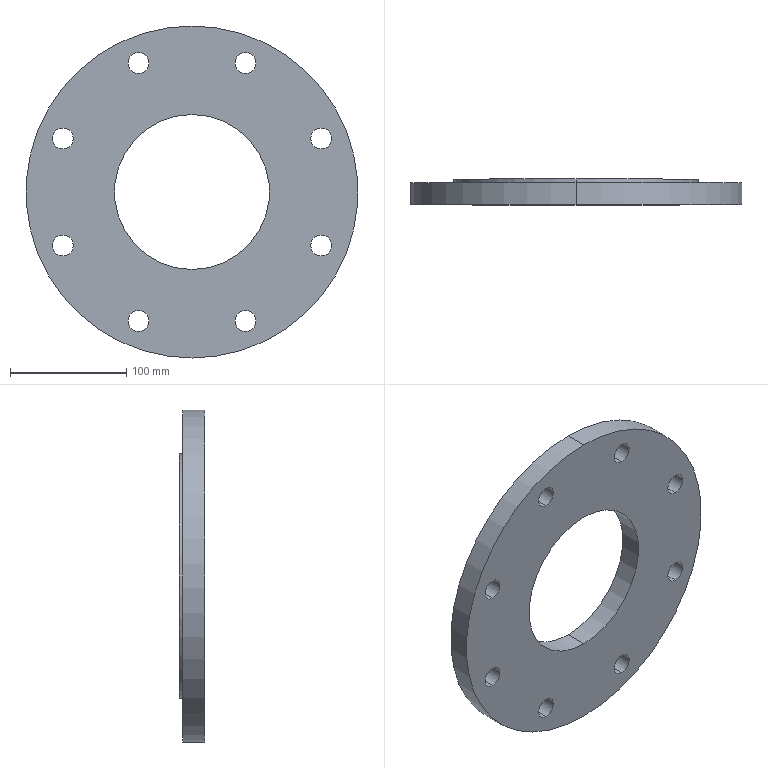Part | SolidWorks | features ICE 2, CirPattern 1, Extrusion 1 | 1 solid | 28 faces | box 285 x 22 x 285 mm | volume 945255 mm3 | cylinder 24 | plane 4 | commonest cylinder face diameters 18 x16 133 x2 170 x2 210 x2 285 x2
STEP:
#1=CARTESIAN_POINT('',(45.922,-9.5,-119.866));
#2=VERTEX_POINT('',#1);
#3=CARTESIAN_POINT('',(45.922,-9.5,-101.866));
#4=VERTEX_POINT('',#3);
#5=CARTESIAN_POINT('',(45.922,-9.5,-110.866));
#6=DIRECTION('',(0.,1.,0.));
#7=DIRECTION('',(-0.7071,0.,0.7071));
#8=AXIS2_PLACEMENT_3D('',#5,#6,#7);
#9=CIRCLE('',#8,9.);
#10=EDGE_CURVE('',#2,#4,#9,.T.);
#11=ORIENTED_EDGE('',*,*,#10,.F.);
#12=CARTESIAN_POINT('',(45.922,9.5,-119.866));
#13=VERTEX_POINT('',#12);
#14=CARTESIAN_POINT('',(45.922,-9.5,-119.866));
#15=DIRECTION('',(0.,1.,0.));
#16=VECTOR('',#15,1000.);
#17=LINE('',#14,#16);
#18=EDGE_CURVE('',#2,#13,#17,.T.);
#19=ORIENTED_EDGE('',*,*,#18,.T.);
#20=CARTESIAN_POINT('',(45.922,9.5,-101.866));
#21=VERTEX_POINT('',#20);
#22=CARTESIAN_POINT('',(45.922,9.5,-110.866));
#23=DIRECTION('',(0.,1.,0.));
#24=DIRECTION('',(-0.7071,0.,0.7071));
#25=AXIS2_PLACEMENT_3D('',#22,#23,#24);
#26=CIRCLE('',#25,9.);
#27=EDGE_CURVE('',#13,#21,#26,.T.);
#28=ORIENTED_EDGE('',*,*,#27,.T.);
#29=CARTESIAN_POINT('',(45.922,-9.5,-101.866));
#30=DIRECTION('',(0.,1.,0.));
#31=VECTOR('',#30,1000.);
#32=LINE('',#29,#31);
#33=EDGE_CURVE('',#4,#21,#32,.T.);
#34=ORIENTED_EDGE('',*,*,#33,.F.);
#35=EDGE_LOOP('',(#11,#19,#28,#34));
#36=FACE_OUTER_BOUND('',#35,.T.);
#37=CARTESIAN_POINT('',(45.922,-9.5,-110.866));
#38=DIRECTION('',(0.,1.,0.));
#39=DIRECTION('',(0.,0.,1.));
#40=AXIS2_PLACEMENT_3D('',#37,#38,#39);
#41=CYLINDRICAL_SURFACE('',#40,9.);
#42=ADVANCED_FACE('',(#36),#41,.F.);
#43=CARTESIAN_POINT('',(110.866,-9.5,-54.922));
#44=VERTEX_POINT('',#43);
#45=CARTESIAN_POINT('',(110.866,-9.5,-36.922));
#46=VERTEX_POINT('',#45);
#47=CARTESIAN_POINT('',(110.866,-9.5,-45.922));
#48=DIRECTION('',(0.,1.,0.));
#49=DIRECTION('',(-1.,0.,0.));
#50=AXIS2_PLACEMENT_3D('',#47,#48,#49);
#51=CIRCLE('',#50,9.);
#52=EDGE_CURVE('',#44,#46,#51,.T.);
#53=ORIENTED_EDGE('',*,*,#52,.F.);
#54=CARTESIAN_POINT('',(110.866,9.5,-54.922));
#55=VERTEX_POINT('',#54);
#56=CARTESIAN_POINT('',(110.866,-9.5,-54.922));
#57=DIRECTION('',(0.,1.,0.));
#58=VECTOR('',#57,1000.);
#59=LINE('',#56,#58);
#60=EDGE_CURVE('',#44,#55,#59,.T.);
#61=ORIENTED_EDGE('',*,*,#60,.T.);
#62=CARTESIAN_POINT('',(110.866,9.5,-36.922));
#63=VERTEX_POINT('',#62);
#64=CARTESIAN_POINT('',(110.866,9.5,-45.922));
#65=DIRECTION('',(0.,1.,0.));
#66=DIRECTION('',(-1.,0.,0.));
#67=AXIS2_PLACEMENT_3D('',#64,#65,#66);
#68=CIRCLE('',#67,9.);
#69=EDGE_CURVE('',#55,#63,#68,.T.);
#70=ORIENTED_EDGE('',*,*,#69,.T.);
#71=CARTESIAN_POINT('',(110.866,-9.5,-36.922));
#72=DIRECTION('',(0.,1.,0.));
#73=VECTOR('',#72,1000.);
#74=LINE('',#71,#73);
#75=EDGE_CURVE('',#46,#63,#74,.T.);
#76=ORIENTED_EDGE('',*,*,#75,.F.);
#77=EDGE_LOOP('',(#53,#61,#70,#76));
#78=FACE_OUTER_BOUND('',#77,.T.);
#79=CARTESIAN_POINT('',(110.866,-9.5,-45.922));
#80=DIRECTION('',(0.,1.,0.));
#81=DIRECTION('',(0.,0.,1.));
#82=AXIS2_PLACEMENT_3D('',#79,#80,#81);
#83=CYLINDRICAL_SURFACE('',#82,9.);
#84=ADVANCED_FACE('',(#78),#83,.F.);
#85=CARTESIAN_POINT('',(110.866,-9.5,36.922));
#86=VERTEX_POINT('',#85);
#87=CARTESIAN_POINT('',(110.866,-9.5,54.922));
#88=VERTEX_POINT('',#87);
#89=CARTESIAN_POINT('',(110.866,-9.5,45.922));
#90=DIRECTION('',(0.,1.,0.));
#91=DIRECTION('',(-0.7071,0.,-0.7071));
#92=AXIS2_PLACEMENT_3D('',#89,#90,#91);
#93=CIRCLE('',#92,9.);
#94=EDGE_CURVE('',#86,#88,#93,.T.);
#95=ORIENTED_EDGE('',*,*,#94,.F.);
#96=CARTESIAN_POINT('',(110.866,9.5,36.922));
#97=VERTEX_POINT('',#96);
#98=CARTESIAN_POINT('',(110.866,-9.5,36.922));
#99=DIRECTION('',(0.,1.,0.));
#100=VECTOR('',#99,1000.);
#101=LINE('',#98,#100);
#102=EDGE_CURVE('',#86,#97,#101,.T.);
#103=ORIENTED_EDGE('',*,*,#102,.T.);
#104=CARTESIAN_POINT('',(110.866,9.5,54.922));
#105=VERTEX_POINT('',#104);
#106=CARTESIAN_POINT('',(110.866,9.5,45.922));
#107=DIRECTION('',(0.,1.,0.));
#108=DIRECTION('',(-0.7071,0.,-0.7071));
#109=AXIS2_PLACEMENT_3D('',#106,#107,#108);
#110=CIRCLE('',#109,9.);
#111=EDGE_CURVE('',#97,#105,#110,.T.);
#112=ORIENTED_EDGE('',*,*,#111,.T.);
#113=CARTESIAN_POINT('',(110.866,-9.5,54.922));
#114=DIRECTION('',(0.,1.,0.));
#115=VECTOR('',#114,1000.);
#116=LINE('',#113,#115);
#117=EDGE_CURVE('',#88,#105,#116,.T.);
#118=ORIENTED_EDGE('',*,*,#117,.F.);
#119=EDGE_LOOP('',(#95,#103,#112,#118));
#120=FACE_OUTER_BOUND('',#119,.T.);
#121=CARTESIAN_POINT('',(110.866,-9.5,45.922));
#122=DIRECTION('',(0.,1.,0.));
#123=DIRECTION('',(0.,0.,1.));
#124=AXIS2_PLACEMENT_3D('',#121,#122,#123);
#125=CYLINDRICAL_SURFACE('',#124,9.);
#126=ADVANCED_FACE('',(#120),#125,.F.);
#127=CARTESIAN_POINT('',(45.922,-9.5,101.866));
#128=VERTEX_POINT('',#127);
#129=CARTESIAN_POINT('',(45.922,-9.5,119.866));
#130=VERTEX_POINT('',#129);
#131=CARTESIAN_POINT('',(45.922,-9.5,110.866));
#132=DIRECTION('',(0.,1.,0.));
#133=DIRECTION('',(0.,0.,-1.));
#134=AXIS2_PLACEMENT_3D('',#131,#132,#133);
#135=CIRCLE('',#134,9.);
#136=EDGE_CURVE('',#128,#130,#135,.T.);
#137=ORIENTED_EDGE('',*,*,#136,.F.);
#138=CARTESIAN_POINT('',(45.922,9.5,101.866));
#139=VERTEX_POINT('',#138);
#140=CARTESIAN_POINT('',(45.922,-9.5,101.866));
#141=DIRECTION('',(0.,1.,0.));
#142=VECTOR('',#141,1000.);
#143=LINE('',#140,#142);
#144=EDGE_CURVE('',#128,#139,#143,.T.);
#145=ORIENTED_EDGE('',*,*,#144,.T.);
#146=CARTESIAN_POINT('',(45.922,9.5,119.866));
#147=VERTEX_POINT('',#146);
#148=CARTESIAN_POINT('',(45.922,9.5,110.866));
#149=DIRECTION('',(0.,1.,0.));
#150=DIRECTION('',(0.,0.,-1.));
#151=AXIS2_PLACEMENT_3D('',#148,#149,#150);
#152=CIRCLE('',#151,9.);
#153=EDGE_CURVE('',#139,#147,#152,.T.);
#154=ORIENTED_EDGE('',*,*,#153,.T.);
#155=CARTESIAN_POINT('',(45.922,-9.5,119.866));
#156=DIRECTION('',(0.,1.,0.));
#157=VECTOR('',#156,1000.);
#158=LINE('',#155,#157);
#159=EDGE_CURVE('',#130,#147,#158,.T.);
#160=ORIENTED_EDGE('',*,*,#159,.F.);
#161=EDGE_LOOP('',(#137,#145,#154,#160));
#162=FACE_OUTER_BOUND('',#161,.T.);
#163=CARTESIAN_POINT('',(45.922,-9.5,110.866));
#164=DIRECTION('',(0.,1.,0.));
#165=DIRECTION('',(0.,0.,1.));
#166=AXIS2_PLACEMENT_3D('',#163,#164,#165);
#167=CYLINDRICAL_SURFACE('',#166,9.);
#168=ADVANCED_FACE('',(#162),#167,.F.);
#169=CARTESIAN_POINT('',(-45.922,-9.5,101.866));
#170=VERTEX_POINT('',#169);
#171=CARTESIAN_POINT('',(-45.922,-9.5,119.866));
#172=VERTEX_POINT('',#171);
#173=CARTESIAN_POINT('',(-45.922,-9.5,110.866));
#174=DIRECTION('',(0.,1.,0.));
#175=DIRECTION('',(0.7071,0.,-0.7071));
#176=AXIS2_PLACEMENT_3D('',#173,#174,#175);
#177=CIRCLE('',#176,9.);
#178=EDGE_CURVE('',#170,#172,#177,.T.);
#179=ORIENTED_EDGE('',*,*,#178,.F.);
#180=CARTESIAN_POINT('',(-45.922,9.5,101.866));
#181=VERTEX_POINT('',#180);
#182=CARTESIAN_POINT('',(-45.922,-9.5,101.866));
#183=DIRECTION('',(0.,1.,0.));
#184=VECTOR('',#183,1000.);
#185=LINE('',#182,#184);
#186=EDGE_CURVE('',#170,#181,#185,.T.);
#187=ORIENTED_EDGE('',*,*,#186,.T.);
#188=CARTESIAN_POINT('',(-45.922,9.5,119.866));
#189=VERTEX_POINT('',#188);
#190=CARTESIAN_POINT('',(-45.922,9.5,110.866));
#191=DIRECTION('',(0.,1.,0.));
#192=DIRECTION('',(0.7071,0.,-0.7071));
#193=AXIS2_PLACEMENT_3D('',#190,#191,#192);
#194=CIRCLE('',#193,9.);
#195=EDGE_CURVE('',#181,#189,#194,.T.);
#196=ORIENTED_EDGE('',*,*,#195,.T.);
#197=CARTESIAN_POINT('',(-45.922,-9.5,119.866));
#198=DIRECTION('',(0.,1.,0.));
#199=VECTOR('',#198,1000.);
#200=LINE('',#197,#199);
#201=EDGE_CURVE('',#172,#189,#200,.T.);
#202=ORIENTED_EDGE('',*,*,#201,.F.);
#203=EDGE_LOOP('',(#179,#187,#196,#202));
#204=FACE_OUTER_BOUND('',#203,.T.);
#205=CARTESIAN_POINT('',(-45.922,-9.5,110.866));
#206=DIRECTION('',(0.,1.,0.));
#207=DIRECTION('',(0.,0.,1.));
#208=AXIS2_PLACEMENT_3D('',#205,#206,#207);
#209=CYLINDRICAL_SURFACE('',#208,9.);
#210=ADVANCED_FACE('',(#204),#209,.F.);
#211=CARTESIAN_POINT('',(-110.866,-9.5,36.922));
#212=VERTEX_POINT('',#211);
#213=CARTESIAN_POINT('',(-110.866,-9.5,54.922));
#214=VERTEX_POINT('',#213);
#215=CARTESIAN_POINT('',(-110.866,-9.5,45.922));
#216=DIRECTION('',(0.,1.,0.));
#217=DIRECTION('',(1.,0.,0.));
#218=AXIS2_PLACEMENT_3D('',#215,#216,#217);
#219=CIRCLE('',#218,9.);
#220=EDGE_CURVE('',#212,#214,#219,.T.);
#221=ORIENTED_EDGE('',*,*,#220,.F.);
#222=CARTESIAN_POINT('',(-110.866,9.5,36.922));
#223=VERTEX_POINT('',#222);
#224=CARTESIAN_POINT('',(-110.866,-9.5,36.922));
#225=DIRECTION('',(0.,1.,0.));
#226=VECTOR('',#225,1000.);
#227=LINE('',#224,#226);
#228=EDGE_CURVE('',#212,#223,#227,.T.);
#229=ORIENTED_EDGE('',*,*,#228,.T.);
#230=CARTESIAN_POINT('',(-110.866,9.5,54.922));
#231=VERTEX_POINT('',#230);
#232=CARTESIAN_POINT('',(-110.866,9.5,45.922));
#233=DIRECTION('',(0.,1.,0.));
#234=DIRECTION('',(1.,0.,0.));
#235=AXIS2_PLACEMENT_3D('',#232,#233,#234);
#236=CIRCLE('',#235,9.);
#237=EDGE_CURVE('',#223,#231,#236,.T.);
#238=ORIENTED_EDGE('',*,*,#237,.T.);
#239=CARTESIAN_POINT('',(-110.866,-9.5,54.922));
#240=DIRECTION('',(0.,1.,0.));
#241=VECTOR('',#240,1000.);
#242=LINE('',#239,#241);
#243=EDGE_CURVE('',#214,#231,#242,.T.);
#244=ORIENTED_EDGE('',*,*,#243,.F.);
#245=EDGE_LOOP('',(#221,#229,#238,#244));
#246=FACE_OUTER_BOUND('',#245,.T.);
#247=CARTESIAN_POINT('',(-110.866,-9.5,45.922));
#248=DIRECTION('',(0.,1.,0.));
#249=DIRECTION('',(0.,0.,1.));
#250=AXIS2_PLACEMENT_3D('',#247,#248,#249);
#251=CYLINDRICAL_SURFACE('',#250,9.);
#252=ADVANCED_FACE('',(#246),#251,.F.);
#253=CARTESIAN_POINT('',(-110.866,-9.5,-54.922));
#254=VERTEX_POINT('',#253);
#255=CARTESIAN_POINT('',(-110.866,-9.5,-36.922));
#256=VERTEX_POINT('',#255);
#257=CARTESIAN_POINT('',(-110.866,-9.5,-45.922));
#258=DIRECTION('',(0.,1.,0.));
#259=DIRECTION('',(0.7071,0.,0.7071));
#260=AXIS2_PLACEMENT_3D('',#257,#258,#259);
#261=CIRCLE('',#260,9.);
#262=EDGE_CURVE('',#254,#256,#261,.T.);
#263=ORIENTED_EDGE('',*,*,#262,.F.);
#264=CARTESIAN_POINT('',(-110.866,9.5,-54.922));
#265=VERTEX_POINT('',#264);
#266=CARTESIAN_POINT('',(-110.866,-9.5,-54.922));
#267=DIRECTION('',(0.,1.,0.));
#268=VECTOR('',#267,1000.);
#269=LINE('',#266,#268);
#270=EDGE_CURVE('',#254,#265,#269,.T.);
#271=ORIENTED_EDGE('',*,*,#270,.T.);
#272=CARTESIAN_POINT('',(-110.866,9.5,-36.922));
#273=VERTEX_POINT('',#272);
#274=CARTESIAN_POINT('',(-110.866,9.5,-45.922));
#275=DIRECTION('',(0.,1.,0.));
#276=DIRECTION('',(0.7071,0.,0.7071));
#277=AXIS2_PLACEMENT_3D('',#274,#275,#276);
#278=CIRCLE('',#277,9.);
#279=EDGE_CURVE('',#265,#273,#278,.T.);
#280=ORIENTED_EDGE('',*,*,#279,.T.);
#281=CARTESIAN_POINT('',(-110.866,-9.5,-36.922));
#282=DIRECTION('',(0.,1.,0.));
#283=VECTOR('',#282,1000.);
#284=LINE('',#281,#283);
#285=EDGE_CURVE('',#256,#273,#284,.T.);
#286=ORIENTED_EDGE('',*,*,#285,.F.);
#287=EDGE_LOOP('',(#263,#271,#280,#286));
#288=FACE_OUTER_BOUND('',#287,.T.);
#289=CARTESIAN_POINT('',(-110.866,-9.5,-45.922));
#290=DIRECTION('',(0.,1.,0.));
#291=DIRECTION('',(0.,0.,1.));
#292=AXIS2_PLACEMENT_3D('',#289,#290,#291);
#293=CYLINDRICAL_SURFACE('',#292,9.);
#294=ADVANCED_FACE('',(#288),#293,.F.);
#295=CARTESIAN_POINT('',(-45.922,-9.5,-119.866));
#296=VERTEX_POINT('',#295);
#297=CARTESIAN_POINT('',(-45.922,-9.5,-101.866));
#298=VERTEX_POINT('',#297);
#299=CARTESIAN_POINT('',(-45.922,-9.5,-110.866));
#300=DIRECTION('',(0.,1.,0.));
#301=DIRECTION('',(0.,0.,1.));
#302=AXIS2_PLACEMENT_3D('',#299,#300,#301);
#303=CIRCLE('',#302,9.);
#304=EDGE_CURVE('',#296,#298,#303,.T.);
#305=ORIENTED_EDGE('',*,*,#304,.F.);
#306=CARTESIAN_POINT('',(-45.922,9.5,-119.866));
#307=VERTEX_POINT('',#306);
#308=CARTESIAN_POINT('',(-45.922,-9.5,-119.866));
#309=DIRECTION('',(0.,1.,0.));
#310=VECTOR('',#309,1000.);
#311=LINE('',#308,#310);
#312=EDGE_CURVE('',#296,#307,#311,.T.);
#313=ORIENTED_EDGE('',*,*,#312,.T.);
#314=CARTESIAN_POINT('',(-45.922,9.5,-101.866));
#315=VERTEX_POINT('',#314);
#316=CARTESIAN_POINT('',(-45.922,9.5,-110.866));
#317=DIRECTION('',(0.,1.,0.));
#318=DIRECTION('',(0.,0.,1.));
#319=AXIS2_PLACEMENT_3D('',#316,#317,#318);
#320=CIRCLE('',#319,9.);
#321=EDGE_CURVE('',#307,#315,#320,.T.);
#322=ORIENTED_EDGE('',*,*,#321,.T.);
#323=CARTESIAN_POINT('',(-45.922,-9.5,-101.866));
#324=DIRECTION('',(0.,1.,0.));
#325=VECTOR('',#324,1000.);
#326=LINE('',#323,#325);
#327=EDGE_CURVE('',#298,#315,#326,.T.);
#328=ORIENTED_EDGE('',*,*,#327,.F.);
#329=EDGE_LOOP('',(#305,#313,#322,#328));
#330=FACE_OUTER_BOUND('',#329,.T.);
#331=CARTESIAN_POINT('',(-45.922,-9.5,-110.866));
#332=DIRECTION('',(0.,1.,0.));
#333=DIRECTION('',(0.,0.,1.));
#334=AXIS2_PLACEMENT_3D('',#331,#332,#333);
#335=CYLINDRICAL_SURFACE('',#334,9.);
#336=ADVANCED_FACE('',(#330),#335,.F.);
#337=CARTESIAN_POINT('',(0.,12.5,-85.));
#338=VERTEX_POINT('',#337);
#339=CARTESIAN_POINT('',(0.,12.5,85.));
#340=VERTEX_POINT('',#339);
#341=CARTESIAN_POINT('',(0.,12.5,0.));
#342=DIRECTION('',(0.,1.,0.));
#343=DIRECTION('',(0.,0.,1.));
#344=AXIS2_PLACEMENT_3D('',#341,#342,#343);
#345=CIRCLE('',#344,85.);
#346=EDGE_CURVE('',#338,#340,#345,.T.);
#347=ORIENTED_EDGE('',*,*,#346,.T.);
#348=CARTESIAN_POINT('',(0.,9.5,85.));
#349=VERTEX_POINT('',#348);
#350=CARTESIAN_POINT('',(0.,12.5,85.));
#351=DIRECTION('',(0.,-1.,0.));
#352=VECTOR('',#351,1000.);
#353=LINE('',#350,#352);
#354=EDGE_CURVE('',#340,#349,#353,.T.);
#355=ORIENTED_EDGE('',*,*,#354,.T.);
#356=CARTESIAN_POINT('',(0.,9.5,-85.));
#357=VERTEX_POINT('',#356);
#358=CARTESIAN_POINT('',(0.,9.5,0.));
#359=DIRECTION('',(0.,-1.,0.));
#360=DIRECTION('',(0.,0.,1.));
#361=AXIS2_PLACEMENT_3D('',#358,#359,#360);
#362=CIRCLE('',#361,85.);
#363=EDGE_CURVE('',#349,#357,#362,.T.);
#364=ORIENTED_EDGE('',*,*,#363,.T.);
#365=CARTESIAN_POINT('',(0.,12.5,-85.));
#366=DIRECTION('',(0.,-1.,0.));
#367=VECTOR('',#366,1000.);
#368=LINE('',#365,#367);
#369=EDGE_CURVE('',#338,#357,#368,.T.);
#370=ORIENTED_EDGE('',*,*,#369,.F.);
#371=EDGE_LOOP('',(#347,#355,#364,#370));
#372=FACE_OUTER_BOUND('',#371,.T.);
#373=CARTESIAN_POINT('',(0.,12.5,0.));
#374=DIRECTION('',(0.,-1.,0.));
#375=DIRECTION('',(0.,0.,-1.));
#376=AXIS2_PLACEMENT_3D('',#373,#374,#375);
#377=CYLINDRICAL_SURFACE('',#376,85.);
#378=ADVANCED_FACE('',(#372),#377,.F.);
#379=CARTESIAN_POINT('',(0.,12.5,105.));
#380=VERTEX_POINT('',#379);
#381=CARTESIAN_POINT('',(0.,12.5,-105.));
#382=VERTEX_POINT('',#381);
#383=CARTESIAN_POINT('',(0.,12.5,0.));
#384=DIRECTION('',(0.,1.,0.));
#385=DIRECTION('',(0.,0.,1.));
#386=AXIS2_PLACEMENT_3D('',#383,#384,#385);
#387=CIRCLE('',#386,105.);
#388=EDGE_CURVE('',#380,#382,#387,.T.);
#389=ORIENTED_EDGE('',*,*,#388,.F.);
#390=CARTESIAN_POINT('',(0.,9.5,105.));
#391=VERTEX_POINT('',#390);
#392=CARTESIAN_POINT('',(0.,12.5,105.));
#393=DIRECTION('',(0.,-1.,0.));
#394=VECTOR('',#393,1000.);
#395=LINE('',#392,#394);
#396=EDGE_CURVE('',#380,#391,#395,.T.);
#397=ORIENTED_EDGE('',*,*,#396,.T.);
#398=CARTESIAN_POINT('',(0.,9.5,-105.));
#399=VERTEX_POINT('',#398);
#400=CARTESIAN_POINT('',(0.,9.5,0.));
#401=DIRECTION('',(0.,1.,0.));
#402=DIRECTION('',(0.,0.,1.));
#403=AXIS2_PLACEMENT_3D('',#400,#401,#402);
#404=CIRCLE('',#403,105.);
#405=EDGE_CURVE('',#391,#399,#404,.T.);
#406=ORIENTED_EDGE('',*,*,#405,.T.);
#407=CARTESIAN_POINT('',(0.,12.5,-105.));
#408=DIRECTION('',(0.,-1.,0.));
#409=VECTOR('',#408,1000.);
#410=LINE('',#407,#409);
#411=EDGE_CURVE('',#382,#399,#410,.T.);
#412=ORIENTED_EDGE('',*,*,#411,.F.);
#413=EDGE_LOOP('',(#389,#397,#406,#412));
#414=FACE_OUTER_BOUND('',#413,.T.);
#415=CARTESIAN_POINT('',(0.,12.5,0.));
#416=DIRECTION('',(0.,-1.,0.));
#417=DIRECTION('',(0.,0.,-1.));
#418=AXIS2_PLACEMENT_3D('',#415,#416,#417);
#419=CYLINDRICAL_SURFACE('',#418,105.);
#420=ADVANCED_FACE('',(#414),#419,.T.);
#421=CARTESIAN_POINT('',(0.,9.5,-66.5));
#422=VERTEX_POINT('',#421);
#423=CARTESIAN_POINT('',(0.,9.5,66.5));
#424=VERTEX_POINT('',#423);
#425=CARTESIAN_POINT('',(0.,9.5,0.));
#426=DIRECTION('',(0.,1.,0.));
#427=DIRECTION('',(0.,0.,1.));
#428=AXIS2_PLACEMENT_3D('',#425,#426,#427);
#429=CIRCLE('',#428,66.5);
#430=EDGE_CURVE('',#422,#424,#429,.T.);
#431=ORIENTED_EDGE('',*,*,#430,.T.);
#432=CARTESIAN_POINT('',(0.,-9.5,66.5));
#433=VERTEX_POINT('',#432);
#434=CARTESIAN_POINT('',(0.,9.5,66.5));
#435=DIRECTION('',(0.,-1.,0.));
#436=VECTOR('',#435,1000.);
#437=LINE('',#434,#436);
#438=EDGE_CURVE('',#424,#433,#437,.T.);
#439=ORIENTED_EDGE('',*,*,#438,.T.);
#440=CARTESIAN_POINT('',(0.,-9.5,-66.5));
#441=VERTEX_POINT('',#440);
#442=CARTESIAN_POINT('',(0.,-9.5,0.));
#443=DIRECTION('',(0.,1.,0.));
#444=DIRECTION('',(0.,0.,1.));
#445=AXIS2_PLACEMENT_3D('',#442,#443,#444);
#446=CIRCLE('',#445,66.5);
#447=EDGE_CURVE('',#441,#433,#446,.T.);
#448=ORIENTED_EDGE('',*,*,#447,.F.);
#449=CARTESIAN_POINT('',(0.,9.5,-66.5));
#450=DIRECTION('',(0.,-1.,0.));
#451=VECTOR('',#450,1000.);
#452=LINE('',#449,#451);
#453=EDGE_CURVE('',#422,#441,#452,.T.);
#454=ORIENTED_EDGE('',*,*,#453,.F.);
#455=EDGE_LOOP('',(#431,#439,#448,#454));
#456=FACE_OUTER_BOUND('',#455,.T.);
#457=CARTESIAN_POINT('',(0.,9.5,0.));
#458=DIRECTION('',(0.,-1.,0.));
#459=DIRECTION('',(0.,0.,-1.));
#460=AXIS2_PLACEMENT_3D('',#457,#458,#459);
#461=CYLINDRICAL_SURFACE('',#460,66.5);
#462=ADVANCED_FACE('',(#456),#461,.F.);
#463=CARTESIAN_POINT('',(0.,9.5,142.5));
#464=VERTEX_POINT('',#463);
#465=CARTESIAN_POINT('',(0.,9.5,-142.5));
#466=VERTEX_POINT('',#465);
#467=CARTESIAN_POINT('',(0.,9.5,0.));
#468=DIRECTION('',(0.,1.,0.));
#469=DIRECTION('',(0.,0.,1.));
#470=AXIS2_PLACEMENT_3D('',#467,#468,#469);
#471=CIRCLE('',#470,142.5);
#472=EDGE_CURVE('',#464,#466,#471,.T.);
#473=ORIENTED_EDGE('',*,*,#472,.F.);
#474=CARTESIAN_POINT('',(0.,-9.5,142.5));
#475=VERTEX_POINT('',#474);
#476=CARTESIAN_POINT('',(0.,9.5,142.5));
#477=DIRECTION('',(0.,-1.,0.));
#478=VECTOR('',#477,1000.);
#479=LINE('',#476,#478);
#480=EDGE_CURVE('',#464,#475,#479,.T.);
#481=ORIENTED_EDGE('',*,*,#480,.T.);
#482=CARTESIAN_POINT('',(0.,-9.5,-142.5));
#483=VERTEX_POINT('',#482);
#484=CARTESIAN_POINT('',(0.,-9.5,0.));
#485=DIRECTION('',(0.,1.,0.));
#486=DIRECTION('',(0.,0.,1.));
#487=AXIS2_PLACEMENT_3D('',#484,#485,#486);
#488=CIRCLE('',#487,142.5);
#489=EDGE_CURVE('',#475,#483,#488,.T.);
#490=ORIENTED_EDGE('',*,*,#489,.T.);
#491=CARTESIAN_POINT('',(0.,9.5,-142.5));
#492=DIRECTION('',(0.,-1.,0.));
#493=VECTOR('',#492,1000.);
#494=LINE('',#491,#493);
#495=EDGE_CURVE('',#466,#483,#494,.T.);
#496=ORIENTED_EDGE('',*,*,#495,.F.);
#497=EDGE_LOOP('',(#473,#481,#490,#496));
#498=FACE_OUTER_BOUND('',#497,.T.);
#499=CARTESIAN_POINT('',(0.,9.5,0.));
#500=DIRECTION('',(0.,-1.,0.));
#501=DIRECTION('',(0.,0.,-1.));
#502=AXIS2_PLACEMENT_3D('',#499,#500,#501);
#503=CYLINDRICAL_SURFACE('',#502,142.5);
#504=ADVANCED_FACE('',(#498),#503,.T.);
#505=ORIENTED_EDGE('',*,*,#430,.F.);
#506=CARTESIAN_POINT('',(0.,9.5,0.));
#507=DIRECTION('',(0.,1.,0.));
#508=DIRECTION('',(0.,0.,1.));
#509=AXIS2_PLACEMENT_3D('',#506,#507,#508);
#510=CIRCLE('',#509,66.5);
#511=EDGE_CURVE('',#424,#422,#510,.T.);
#512=ORIENTED_EDGE('',*,*,#511,.F.);
#513=EDGE_LOOP('',(#505,#512));
#514=FACE_BOUND('',#513,.T.);
#515=CARTESIAN_POINT('',(0.,9.5,0.));
#516=DIRECTION('',(0.,-1.,0.));
#517=DIRECTION('',(0.,0.,1.));
#518=AXIS2_PLACEMENT_3D('',#515,#516,#517);
#519=CIRCLE('',#518,85.);
#520=EDGE_CURVE('',#357,#349,#519,.T.);
#521=ORIENTED_EDGE('',*,*,#520,.F.);
#522=ORIENTED_EDGE('',*,*,#363,.F.);
#523=EDGE_LOOP('',(#521,#522));
#524=FACE_OUTER_BOUND('',#523,.T.);
#525=CARTESIAN_POINT('',(0.,9.5,0.));
#526=DIRECTION('',(0.,1.,0.));
#527=DIRECTION('',(0.,0.,1.));
#528=AXIS2_PLACEMENT_3D('',#525,#526,#527);
#529=PLANE('',#528);
#530=ADVANCED_FACE('',(#514,#524),#529,.T.);
#531=CARTESIAN_POINT('',(45.922,9.5,-110.866));
#532=DIRECTION('',(0.,1.,0.));
#533=DIRECTION('',(-0.7071,0.,0.7071));
#534=AXIS2_PLACEMENT_3D('',#531,#532,#533);
#535=CIRCLE('',#534,9.);
#536=EDGE_CURVE('',#21,#13,#535,.T.);
#537=ORIENTED_EDGE('',*,*,#536,.F.);
#538=ORIENTED_EDGE('',*,*,#27,.F.);
#539=EDGE_LOOP('',(#537,#538));
#540=FACE_BOUND('',#539,.T.);
#541=CARTESIAN_POINT('',(110.866,9.5,-45.922));
#542=DIRECTION('',(0.,1.,0.));
#543=DIRECTION('',(-1.,0.,0.));
#544=AXIS2_PLACEMENT_3D('',#541,#542,#543);
#545=CIRCLE('',#544,9.);
#546=EDGE_CURVE('',#63,#55,#545,.T.);
#547=ORIENTED_EDGE('',*,*,#546,.F.);
#548=ORIENTED_EDGE('',*,*,#69,.F.);
#549=EDGE_LOOP('',(#547,#548));
#550=FACE_BOUND('',#549,.T.);
#551=CARTESIAN_POINT('',(110.866,9.5,45.922));
#552=DIRECTION('',(0.,1.,0.));
#553=DIRECTION('',(-0.7071,0.,-0.7071));
#554=AXIS2_PLACEMENT_3D('',#551,#552,#553);
#555=CIRCLE('',#554,9.);
#556=EDGE_CURVE('',#105,#97,#555,.T.);
#557=ORIENTED_EDGE('',*,*,#556,.F.);
#558=ORIENTED_EDGE('',*,*,#111,.F.);
#559=EDGE_LOOP('',(#557,#558));
#560=FACE_BOUND('',#559,.T.);
#561=CARTESIAN_POINT('',(45.922,9.5,110.866));
#562=DIRECTION('',(0.,1.,0.));
#563=DIRECTION('',(0.,0.,-1.));
#564=AXIS2_PLACEMENT_3D('',#561,#562,#563);
#565=CIRCLE('',#564,9.);
#566=EDGE_CURVE('',#147,#139,#565,.T.);
#567=ORIENTED_EDGE('',*,*,#566,.F.);
#568=ORIENTED_EDGE('',*,*,#153,.F.);
#569=EDGE_LOOP('',(#567,#568));
#570=FACE_BOUND('',#569,.T.);
#571=CARTESIAN_POINT('',(-45.922,9.5,110.866));
#572=DIRECTION('',(0.,1.,0.));
#573=DIRECTION('',(0.7071,0.,-0.7071));
#574=AXIS2_PLACEMENT_3D('',#571,#572,#573);
#575=CIRCLE('',#574,9.);
#576=EDGE_CURVE('',#189,#181,#575,.T.);
#577=ORIENTED_EDGE('',*,*,#576,.F.);
#578=ORIENTED_EDGE('',*,*,#195,.F.);
#579=EDGE_LOOP('',(#577,#578));
#580=FACE_BOUND('',#579,.T.);
#581=CARTESIAN_POINT('',(-110.866,9.5,45.922));
#582=DIRECTION('',(0.,1.,0.));
#583=DIRECTION('',(1.,0.,0.));
#584=AXIS2_PLACEMENT_3D('',#581,#582,#583);
#585=CIRCLE('',#584,9.);
#586=EDGE_CURVE('',#231,#223,#585,.T.);
#587=ORIENTED_EDGE('',*,*,#586,.F.);
#588=ORIENTED_EDGE('',*,*,#237,.F.);
#589=EDGE_LOOP('',(#587,#588));
#590=FACE_BOUND('',#589,.T.);
#591=CARTESIAN_POINT('',(-110.866,9.5,-45.922));
#592=DIRECTION('',(0.,1.,0.));
#593=DIRECTION('',(0.7071,0.,0.7071));
#594=AXIS2_PLACEMENT_3D('',#591,#592,#593);
#595=CIRCLE('',#594,9.);
#596=EDGE_CURVE('',#273,#265,#595,.T.);
#597=ORIENTED_EDGE('',*,*,#596,.F.);
#598=ORIENTED_EDGE('',*,*,#279,.F.);
#599=EDGE_LOOP('',(#597,#598));
#600=FACE_BOUND('',#599,.T.);
#601=CARTESIAN_POINT('',(-45.922,9.5,-110.866));
#602=DIRECTION('',(0.,1.,0.));
#603=DIRECTION('',(0.,0.,1.));
#604=AXIS2_PLACEMENT_3D('',#601,#602,#603);
#605=CIRCLE('',#604,9.);
#606=EDGE_CURVE('',#315,#307,#605,.T.);
#607=ORIENTED_EDGE('',*,*,#606,.F.);
#608=ORIENTED_EDGE('',*,*,#321,.F.);
#609=EDGE_LOOP('',(#607,#608));
#610=FACE_BOUND('',#609,.T.);
#611=CARTESIAN_POINT('',(0.,9.5,0.));
#612=DIRECTION('',(0.,1.,0.));
#613=DIRECTION('',(0.,0.,1.));
#614=AXIS2_PLACEMENT_3D('',#611,#612,#613);
#615=CIRCLE('',#614,105.);
#616=EDGE_CURVE('',#399,#391,#615,.T.);
#617=ORIENTED_EDGE('',*,*,#616,.F.);
#618=ORIENTED_EDGE('',*,*,#405,.F.);
#619=EDGE_LOOP('',(#617,#618));
#620=FACE_BOUND('',#619,.T.);
#621=CARTESIAN_POINT('',(0.,9.5,0.));
#622=DIRECTION('',(0.,1.,0.));
#623=DIRECTION('',(0.,0.,1.));
#624=AXIS2_PLACEMENT_3D('',#621,#622,#623);
#625=CIRCLE('',#624,142.5);
#626=EDGE_CURVE('',#466,#464,#625,.T.);
#627=ORIENTED_EDGE('',*,*,#626,.T.);
#628=ORIENTED_EDGE('',*,*,#472,.T.);
#629=EDGE_LOOP('',(#627,#628));
#630=FACE_OUTER_BOUND('',#629,.T.);
#631=CARTESIAN_POINT('',(0.,9.5,0.));
#632=DIRECTION('',(0.,1.,0.));
#633=DIRECTION('',(0.,0.,1.));
#634=AXIS2_PLACEMENT_3D('',#631,#632,#633);
#635=PLANE('',#634);
#636=ADVANCED_FACE('',(#540,#550,#560,#570,#580,#590,#600,#610,#620,#630),#635,.T.);
#637=CARTESIAN_POINT('',(45.922,-9.5,-110.866));
#638=DIRECTION('',(0.,1.,0.));
#639=DIRECTION('',(-0.7071,0.,0.7071));
#640=AXIS2_PLACEMENT_3D('',#637,#638,#639);
#641=CIRCLE('',#640,9.);
#642=EDGE_CURVE('',#4,#2,#641,.T.);
#643=ORIENTED_EDGE('',*,*,#642,.T.);
#644=ORIENTED_EDGE('',*,*,#10,.T.);
#645=EDGE_LOOP('',(#643,#644));
#646=FACE_BOUND('',#645,.T.);
#647=CARTESIAN_POINT('',(110.866,-9.5,-45.922));
#648=DIRECTION('',(0.,1.,0.));
#649=DIRECTION('',(-1.,0.,0.));
#650=AXIS2_PLACEMENT_3D('',#647,#648,#649);
#651=CIRCLE('',#650,9.);
#652=EDGE_CURVE('',#46,#44,#651,.T.);
#653=ORIENTED_EDGE('',*,*,#652,.T.);
#654=ORIENTED_EDGE('',*,*,#52,.T.);
#655=EDGE_LOOP('',(#653,#654));
#656=FACE_BOUND('',#655,.T.);
#657=CARTESIAN_POINT('',(110.866,-9.5,45.922));
#658=DIRECTION('',(0.,1.,0.));
#659=DIRECTION('',(-0.7071,0.,-0.7071));
#660=AXIS2_PLACEMENT_3D('',#657,#658,#659);
#661=CIRCLE('',#660,9.);
#662=EDGE_CURVE('',#88,#86,#661,.T.);
#663=ORIENTED_EDGE('',*,*,#662,.T.);
#664=ORIENTED_EDGE('',*,*,#94,.T.);
#665=EDGE_LOOP('',(#663,#664));
#666=FACE_BOUND('',#665,.T.);
#667=CARTESIAN_POINT('',(45.922,-9.5,110.866));
#668=DIRECTION('',(0.,1.,0.));
#669=DIRECTION('',(0.,0.,-1.));
#670=AXIS2_PLACEMENT_3D('',#667,#668,#669);
#671=CIRCLE('',#670,9.);
#672=EDGE_CURVE('',#130,#128,#671,.T.);
#673=ORIENTED_EDGE('',*,*,#672,.T.);
#674=ORIENTED_EDGE('',*,*,#136,.T.);
#675=EDGE_LOOP('',(#673,#674));
#676=FACE_BOUND('',#675,.T.);
#677=CARTESIAN_POINT('',(-45.922,-9.5,110.866));
#678=DIRECTION('',(0.,1.,0.));
#679=DIRECTION('',(0.7071,0.,-0.7071));
#680=AXIS2_PLACEMENT_3D('',#677,#678,#679);
#681=CIRCLE('',#680,9.);
#682=EDGE_CURVE('',#172,#170,#681,.T.);
#683=ORIENTED_EDGE('',*,*,#682,.T.);
#684=ORIENTED_EDGE('',*,*,#178,.T.);
#685=EDGE_LOOP('',(#683,#684));
#686=FACE_BOUND('',#685,.T.);
#687=CARTESIAN_POINT('',(-110.866,-9.5,45.922));
#688=DIRECTION('',(0.,1.,0.));
#689=DIRECTION('',(1.,0.,0.));
#690=AXIS2_PLACEMENT_3D('',#687,#688,#689);
#691=CIRCLE('',#690,9.);
#692=EDGE_CURVE('',#214,#212,#691,.T.);
#693=ORIENTED_EDGE('',*,*,#692,.T.);
#694=ORIENTED_EDGE('',*,*,#220,.T.);
#695=EDGE_LOOP('',(#693,#694));
#696=FACE_BOUND('',#695,.T.);
#697=CARTESIAN_POINT('',(-110.866,-9.5,-45.922));
#698=DIRECTION('',(0.,1.,0.));
#699=DIRECTION('',(0.7071,0.,0.7071));
#700=AXIS2_PLACEMENT_3D('',#697,#698,#699);
#701=CIRCLE('',#700,9.);
#702=EDGE_CURVE('',#256,#254,#701,.T.);
#703=ORIENTED_EDGE('',*,*,#702,.T.);
#704=ORIENTED_EDGE('',*,*,#262,.T.);
#705=EDGE_LOOP('',(#703,#704));
#706=FACE_BOUND('',#705,.T.);
#707=CARTESIAN_POINT('',(-45.922,-9.5,-110.866));
#708=DIRECTION('',(0.,1.,0.));
#709=DIRECTION('',(0.,0.,1.));
#710=AXIS2_PLACEMENT_3D('',#707,#708,#709);
#711=CIRCLE('',#710,9.);
#712=EDGE_CURVE('',#298,#296,#711,.T.);
#713=ORIENTED_EDGE('',*,*,#712,.T.);
#714=ORIENTED_EDGE('',*,*,#304,.T.);
#715=EDGE_LOOP('',(#713,#714));
#716=FACE_BOUND('',#715,.T.);
#717=CARTESIAN_POINT('',(0.,-9.5,0.));
#718=DIRECTION('',(0.,1.,0.));
#719=DIRECTION('',(0.,0.,1.));
#720=AXIS2_PLACEMENT_3D('',#717,#718,#719);
#721=CIRCLE('',#720,142.5);
#722=EDGE_CURVE('',#483,#475,#721,.T.);
#723=ORIENTED_EDGE('',*,*,#722,.F.);
#724=ORIENTED_EDGE('',*,*,#489,.F.);
#725=EDGE_LOOP('',(#723,#724));
#726=FACE_OUTER_BOUND('',#725,.T.);
#727=ORIENTED_EDGE('',*,*,#447,.T.);
#728=CARTESIAN_POINT('',(0.,-9.5,0.));
#729=DIRECTION('',(0.,1.,0.));
#730=DIRECTION('',(0.,0.,1.));
#731=AXIS2_PLACEMENT_3D('',#728,#729,#730);
#732=CIRCLE('',#731,66.5);
#733=EDGE_CURVE('',#433,#441,#732,.T.);
#734=ORIENTED_EDGE('',*,*,#733,.T.);
#735=EDGE_LOOP('',(#727,#734));
#736=FACE_BOUND('',#735,.T.);
#737=CARTESIAN_POINT('',(0.,-9.5,0.));
#738=DIRECTION('',(0.,1.,0.));
#739=DIRECTION('',(0.,0.,1.));
#740=AXIS2_PLACEMENT_3D('',#737,#738,#739);
#741=PLANE('',#740);
#742=ADVANCED_FACE('',(#646,#656,#666,#676,#686,#696,#706,#716,#726,#736),#741,.F.);
#743=ORIENTED_EDGE('',*,*,#480,.F.);
#744=ORIENTED_EDGE('',*,*,#626,.F.);
#745=ORIENTED_EDGE('',*,*,#495,.T.);
#746=ORIENTED_EDGE('',*,*,#722,.T.);
#747=EDGE_LOOP('',(#743,#744,#745,#746));
#748=FACE_OUTER_BOUND('',#747,.T.);
#749=CARTESIAN_POINT('',(0.,9.5,0.));
#750=DIRECTION('',(0.,-1.,0.));
#751=DIRECTION('',(0.,0.,-1.));
#752=AXIS2_PLACEMENT_3D('',#749,#750,#751);
#753=CYLINDRICAL_SURFACE('',#752,142.5);
#754=ADVANCED_FACE('',(#748),#753,.T.);
#755=ORIENTED_EDGE('',*,*,#438,.F.);
#756=ORIENTED_EDGE('',*,*,#511,.T.);
#757=ORIENTED_EDGE('',*,*,#453,.T.);
#758=ORIENTED_EDGE('',*,*,#733,.F.);
#759=EDGE_LOOP('',(#755,#756,#757,#758));
#760=FACE_OUTER_BOUND('',#759,.T.);
#761=CARTESIAN_POINT('',(0.,9.5,0.));
#762=DIRECTION('',(0.,-1.,0.));
#763=DIRECTION('',(0.,0.,-1.));
#764=AXIS2_PLACEMENT_3D('',#761,#762,#763);
#765=CYLINDRICAL_SURFACE('',#764,66.5);
#766=ADVANCED_FACE('',(#760),#765,.F.);
#767=CARTESIAN_POINT('',(0.,12.5,0.));
#768=DIRECTION('',(0.,1.,0.));
#769=DIRECTION('',(0.,0.,1.));
#770=AXIS2_PLACEMENT_3D('',#767,#768,#769);
#771=CIRCLE('',#770,105.);
#772=EDGE_CURVE('',#382,#380,#771,.T.);
#773=ORIENTED_EDGE('',*,*,#772,.T.);
#774=ORIENTED_EDGE('',*,*,#388,.T.);
#775=EDGE_LOOP('',(#773,#774));
#776=FACE_OUTER_BOUND('',#775,.T.);
#777=ORIENTED_EDGE('',*,*,#346,.F.);
#778=CARTESIAN_POINT('',(0.,12.5,0.));
#779=DIRECTION('',(0.,1.,0.));
#780=DIRECTION('',(0.,0.,1.));
#781=AXIS2_PLACEMENT_3D('',#778,#779,#780);
#782=CIRCLE('',#781,85.);
#783=EDGE_CURVE('',#340,#338,#782,.T.);
#784=ORIENTED_EDGE('',*,*,#783,.F.);
#785=EDGE_LOOP('',(#777,#784));
#786=FACE_BOUND('',#785,.T.);
#787=CARTESIAN_POINT('',(0.,12.5,0.));
#788=DIRECTION('',(0.,1.,0.));
#789=DIRECTION('',(0.,0.,1.));
#790=AXIS2_PLACEMENT_3D('',#787,#788,#789);
#791=PLANE('',#790);
#792=ADVANCED_FACE('',(#776,#786),#791,.T.);
#793=ORIENTED_EDGE('',*,*,#396,.F.);
#794=ORIENTED_EDGE('',*,*,#772,.F.);
#795=ORIENTED_EDGE('',*,*,#411,.T.);
#796=ORIENTED_EDGE('',*,*,#616,.T.);
#797=EDGE_LOOP('',(#793,#794,#795,#796));
#798=FACE_OUTER_BOUND('',#797,.T.);
#799=CARTESIAN_POINT('',(0.,12.5,0.));
#800=DIRECTION('',(0.,-1.,0.));
#801=DIRECTION('',(0.,0.,-1.));
#802=AXIS2_PLACEMENT_3D('',#799,#800,#801);
#803=CYLINDRICAL_SURFACE('',#802,105.);
#804=ADVANCED_FACE('',(#798),#803,.T.);
#805=ORIENTED_EDGE('',*,*,#354,.F.);
#806=ORIENTED_EDGE('',*,*,#783,.T.);
#807=ORIENTED_EDGE('',*,*,#369,.T.);
#808=ORIENTED_EDGE('',*,*,#520,.T.);
#809=EDGE_LOOP('',(#805,#806,#807,#808));
#810=FACE_OUTER_BOUND('',#809,.T.);
#811=CARTESIAN_POINT('',(0.,12.5,0.));
#812=DIRECTION('',(0.,-1.,0.));
#813=DIRECTION('',(0.,0.,-1.));
#814=AXIS2_PLACEMENT_3D('',#811,#812,#813);
#815=CYLINDRICAL_SURFACE('',#814,85.);
#816=ADVANCED_FACE('',(#810),#815,.F.);
#817=ORIENTED_EDGE('',*,*,#312,.F.);
#818=ORIENTED_EDGE('',*,*,#712,.F.);
#819=ORIENTED_EDGE('',*,*,#327,.T.);
#820=ORIENTED_EDGE('',*,*,#606,.T.);
#821=EDGE_LOOP('',(#817,#818,#819,#820));
#822=FACE_OUTER_BOUND('',#821,.T.);
#823=CARTESIAN_POINT('',(-45.922,-9.5,-110.866));
#824=DIRECTION('',(0.,1.,0.));
#825=DIRECTION('',(0.,0.,1.));
#826=AXIS2_PLACEMENT_3D('',#823,#824,#825);
#827=CYLINDRICAL_SURFACE('',#826,9.);
#828=ADVANCED_FACE('',(#822),#827,.F.);
#829=ORIENTED_EDGE('',*,*,#270,.F.);
#830=ORIENTED_EDGE('',*,*,#702,.F.);
#831=ORIENTED_EDGE('',*,*,#285,.T.);
#832=ORIENTED_EDGE('',*,*,#596,.T.);
#833=EDGE_LOOP('',(#829,#830,#831,#832));
#834=FACE_OUTER_BOUND('',#833,.T.);
#835=CARTESIAN_POINT('',(-110.866,-9.5,-45.922));
#836=DIRECTION('',(0.,1.,0.));
#837=DIRECTION('',(0.,0.,1.));
#838=AXIS2_PLACEMENT_3D('',#835,#836,#837);
#839=CYLINDRICAL_SURFACE('',#838,9.);
#840=ADVANCED_FACE('',(#834),#839,.F.);
#841=ORIENTED_EDGE('',*,*,#228,.F.);
#842=ORIENTED_EDGE('',*,*,#692,.F.);
#843=ORIENTED_EDGE('',*,*,#243,.T.);
#844=ORIENTED_EDGE('',*,*,#586,.T.);
#845=EDGE_LOOP('',(#841,#842,#843,#844));
#846=FACE_OUTER_BOUND('',#845,.T.);
#847=CARTESIAN_POINT('',(-110.866,-9.5,45.922));
#848=DIRECTION('',(0.,1.,0.));
#849=DIRECTION('',(0.,0.,1.));
#850=AXIS2_PLACEMENT_3D('',#847,#848,#849);
#851=CYLINDRICAL_SURFACE('',#850,9.);
#852=ADVANCED_FACE('',(#846),#851,.F.);
#853=ORIENTED_EDGE('',*,*,#186,.F.);
#854=ORIENTED_EDGE('',*,*,#682,.F.);
#855=ORIENTED_EDGE('',*,*,#201,.T.);
#856=ORIENTED_EDGE('',*,*,#576,.T.);
#857=EDGE_LOOP('',(#853,#854,#855,#856));
#858=FACE_OUTER_BOUND('',#857,.T.);
#859=CARTESIAN_POINT('',(-45.922,-9.5,110.866));
#860=DIRECTION('',(0.,1.,0.));
#861=DIRECTION('',(0.,0.,1.));
#862=AXIS2_PLACEMENT_3D('',#859,#860,#861);
#863=CYLINDRICAL_SURFACE('',#862,9.);
#864=ADVANCED_FACE('',(#858),#863,.F.);
#865=ORIENTED_EDGE('',*,*,#144,.F.);
#866=ORIENTED_EDGE('',*,*,#672,.F.);
#867=ORIENTED_EDGE('',*,*,#159,.T.);
#868=ORIENTED_EDGE('',*,*,#566,.T.);
#869=EDGE_LOOP('',(#865,#866,#867,#868));
#870=FACE_OUTER_BOUND('',#869,.T.);
#871=CARTESIAN_POINT('',(45.922,-9.5,110.866));
#872=DIRECTION('',(0.,1.,0.));
#873=DIRECTION('',(0.,0.,1.));
#874=AXIS2_PLACEMENT_3D('',#871,#872,#873);
#875=CYLINDRICAL_SURFACE('',#874,9.);
#876=ADVANCED_FACE('',(#870),#875,.F.);
#877=ORIENTED_EDGE('',*,*,#102,.F.);
#878=ORIENTED_EDGE('',*,*,#662,.F.);
#879=ORIENTED_EDGE('',*,*,#117,.T.);
#880=ORIENTED_EDGE('',*,*,#556,.T.);
#881=EDGE_LOOP('',(#877,#878,#879,#880));
#882=FACE_OUTER_BOUND('',#881,.T.);
#883=CARTESIAN_POINT('',(110.866,-9.5,45.922));
#884=DIRECTION('',(0.,1.,0.));
#885=DIRECTION('',(0.,0.,1.));
#886=AXIS2_PLACEMENT_3D('',#883,#884,#885);
#887=CYLINDRICAL_SURFACE('',#886,9.);
#888=ADVANCED_FACE('',(#882),#887,.F.);
#889=ORIENTED_EDGE('',*,*,#60,.F.);
#890=ORIENTED_EDGE('',*,*,#652,.F.);
#891=ORIENTED_EDGE('',*,*,#75,.T.);
#892=ORIENTED_EDGE('',*,*,#546,.T.);
#893=EDGE_LOOP('',(#889,#890,#891,#892));
#894=FACE_OUTER_BOUND('',#893,.T.);
#895=CARTESIAN_POINT('',(110.866,-9.5,-45.922));
#896=DIRECTION('',(0.,1.,0.));
#897=DIRECTION('',(0.,0.,1.));
#898=AXIS2_PLACEMENT_3D('',#895,#896,#897);
#899=CYLINDRICAL_SURFACE('',#898,9.);
#900=ADVANCED_FACE('',(#894),#899,.F.);
#901=ORIENTED_EDGE('',*,*,#18,.F.);
#902=ORIENTED_EDGE('',*,*,#642,.F.);
#903=ORIENTED_EDGE('',*,*,#33,.T.);
#904=ORIENTED_EDGE('',*,*,#536,.T.);
#905=EDGE_LOOP('',(#901,#902,#903,#904));
#906=FACE_OUTER_BOUND('',#905,.T.);
#907=CARTESIAN_POINT('',(45.922,-9.5,-110.866));
#908=DIRECTION('',(0.,1.,0.));
#909=DIRECTION('',(0.,0.,1.));
#910=AXIS2_PLACEMENT_3D('',#907,#908,#909);
#911=CYLINDRICAL_SURFACE('',#910,9.);
#912=ADVANCED_FACE('',(#906),#911,.F.);
#913=CLOSED_SHELL('',(#42,#84,#126,#168,#210,#252,#294,#336,#378,#420,#462,#504,#530,#636,#742,#754,#766,#792,#804,#816,#828,#840,#852,#864,#876,#888,#900,#912));
#914=MANIFOLD_SOLID_BREP('',#913);
#915=CARTESIAN_POINT('',(0.,0.,0.));
#916=DIRECTION('',(0.,0.,1.));
#917=DIRECTION('',(1.,0.,0.));
#918=AXIS2_PLACEMENT_3D('',#915,#916,#917);
#919=(LENGTH_UNIT()NAMED_UNIT(*)SI_UNIT(.MILLI.,.METRE.));
#920=UNCERTAINTY_MEASURE_WITH_UNIT(LENGTH_MEASURE(0.00001),#919,'','');
#921=(NAMED_UNIT(*)PLANE_ANGLE_UNIT()SI_UNIT($,.RADIAN.));
#922=(NAMED_UNIT(*)SI_UNIT($,.STERADIAN.)SOLID_ANGLE_UNIT());
#923=(GEOMETRIC_REPRESENTATION_CONTEXT(3)GLOBAL_UNCERTAINTY_ASSIGNED_CONTEXT((#920))GLOBAL_UNIT_ASSIGNED_CONTEXT((#919,#921,#922))REPRESENTATION_CONTEXT('',''));
#924=ADVANCED_BREP_SHAPE_REPRESENTATION('',(#914,#918),#923);